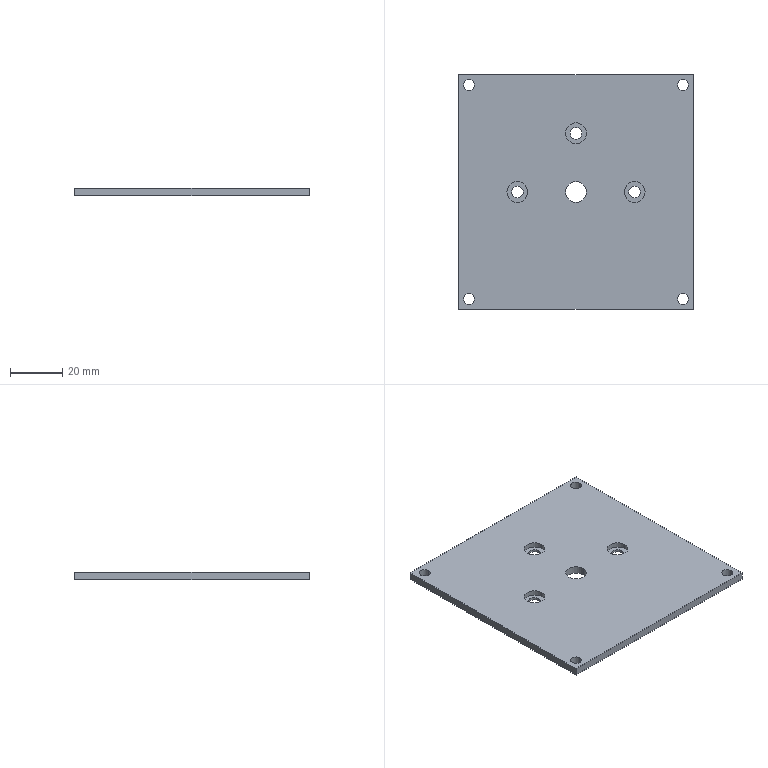Part | STEP file | output terminal base plate^spray gun PTFE model | 1 solid | 31 faces | box 90 x 90 x 3 mm | volume 23634 mm3 | cylinder 22 | plane 9 | commonest cylinder face diameters 4.2 x8 8 x8 4.5 x6
STEP:
#1=CARTESIAN_POINT('',(2.25,22.5,0.));
#2=VERTEX_POINT('',#1);
#3=CARTESIAN_POINT('',(-2.25,22.5,0.));
#4=VERTEX_POINT('',#3);
#5=CARTESIAN_POINT('',(0.,22.5,0.));
#6=DIRECTION('',(0.,0.,-1.));
#7=DIRECTION('',(1.,0.,0.));
#8=AXIS2_PLACEMENT_3D('',#5,#6,#7);
#9=CIRCLE('',#8,2.25);
#10=EDGE_CURVE('',#2,#4,#9,.T.);
#11=ORIENTED_EDGE('',*,*,#10,.T.);
#12=CARTESIAN_POINT('',(-2.25,22.5,1.));
#13=VERTEX_POINT('',#12);
#14=CARTESIAN_POINT('',(-2.25,22.5,-7.));
#15=DIRECTION('',(0.,0.,1.));
#16=VECTOR('',#15,1000.);
#17=LINE('',#14,#16);
#18=EDGE_CURVE('',#4,#13,#17,.T.);
#19=ORIENTED_EDGE('',*,*,#18,.T.);
#20=CARTESIAN_POINT('',(2.25,22.5,1.));
#21=VERTEX_POINT('',#20);
#22=CARTESIAN_POINT('',(0.,22.5,1.));
#23=DIRECTION('',(0.,0.,-1.));
#24=DIRECTION('',(1.,0.,0.));
#25=AXIS2_PLACEMENT_3D('',#22,#23,#24);
#26=CIRCLE('',#25,2.25);
#27=EDGE_CURVE('',#21,#13,#26,.T.);
#28=ORIENTED_EDGE('',*,*,#27,.F.);
#29=CARTESIAN_POINT('',(2.25,22.5,-7.));
#30=DIRECTION('',(0.,0.,1.));
#31=VECTOR('',#30,1000.);
#32=LINE('',#29,#31);
#33=EDGE_CURVE('',#2,#21,#32,.T.);
#34=ORIENTED_EDGE('',*,*,#33,.F.);
#35=EDGE_LOOP('',(#11,#19,#28,#34));
#36=FACE_OUTER_BOUND('',#35,.T.);
#37=CARTESIAN_POINT('',(0.,22.5,-7.));
#38=DIRECTION('',(0.,0.,1.));
#39=DIRECTION('',(1.,0.,0.));
#40=AXIS2_PLACEMENT_3D('',#37,#38,#39);
#41=CYLINDRICAL_SURFACE('',#40,2.25);
#42=ADVANCED_FACE('',(#36),#41,.F.);
#43=CARTESIAN_POINT('',(24.75,0.,0.));
#44=VERTEX_POINT('',#43);
#45=CARTESIAN_POINT('',(20.25,0.,0.));
#46=VERTEX_POINT('',#45);
#47=CARTESIAN_POINT('',(22.5,0.,0.));
#48=DIRECTION('',(0.,0.,-1.));
#49=DIRECTION('',(1.,0.,0.));
#50=AXIS2_PLACEMENT_3D('',#47,#48,#49);
#51=CIRCLE('',#50,2.25);
#52=EDGE_CURVE('',#44,#46,#51,.T.);
#53=ORIENTED_EDGE('',*,*,#52,.T.);
#54=CARTESIAN_POINT('',(20.25,0.,1.));
#55=VERTEX_POINT('',#54);
#56=CARTESIAN_POINT('',(20.25,0.,-7.));
#57=DIRECTION('',(0.,0.,1.));
#58=VECTOR('',#57,1000.);
#59=LINE('',#56,#58);
#60=EDGE_CURVE('',#46,#55,#59,.T.);
#61=ORIENTED_EDGE('',*,*,#60,.T.);
#62=CARTESIAN_POINT('',(24.75,0.,1.));
#63=VERTEX_POINT('',#62);
#64=CARTESIAN_POINT('',(22.5,0.,1.));
#65=DIRECTION('',(0.,0.,-1.));
#66=DIRECTION('',(1.,0.,0.));
#67=AXIS2_PLACEMENT_3D('',#64,#65,#66);
#68=CIRCLE('',#67,2.25);
#69=EDGE_CURVE('',#63,#55,#68,.T.);
#70=ORIENTED_EDGE('',*,*,#69,.F.);
#71=CARTESIAN_POINT('',(24.75,0.,-7.));
#72=DIRECTION('',(0.,0.,1.));
#73=VECTOR('',#72,1000.);
#74=LINE('',#71,#73);
#75=EDGE_CURVE('',#44,#63,#74,.T.);
#76=ORIENTED_EDGE('',*,*,#75,.F.);
#77=EDGE_LOOP('',(#53,#61,#70,#76));
#78=FACE_OUTER_BOUND('',#77,.T.);
#79=CARTESIAN_POINT('',(22.5,0.,-7.));
#80=DIRECTION('',(0.,0.,1.));
#81=DIRECTION('',(1.,0.,0.));
#82=AXIS2_PLACEMENT_3D('',#79,#80,#81);
#83=CYLINDRICAL_SURFACE('',#82,2.25);
#84=ADVANCED_FACE('',(#78),#83,.F.);
#85=CARTESIAN_POINT('',(-20.25,0.,0.));
#86=VERTEX_POINT('',#85);
#87=CARTESIAN_POINT('',(-24.75,0.,0.));
#88=VERTEX_POINT('',#87);
#89=CARTESIAN_POINT('',(-22.5,0.,0.));
#90=DIRECTION('',(0.,0.,-1.));
#91=DIRECTION('',(1.,0.,0.));
#92=AXIS2_PLACEMENT_3D('',#89,#90,#91);
#93=CIRCLE('',#92,2.25);
#94=EDGE_CURVE('',#86,#88,#93,.T.);
#95=ORIENTED_EDGE('',*,*,#94,.T.);
#96=CARTESIAN_POINT('',(-24.75,0.,1.));
#97=VERTEX_POINT('',#96);
#98=CARTESIAN_POINT('',(-24.75,0.,-7.));
#99=DIRECTION('',(0.,0.,1.));
#100=VECTOR('',#99,1000.);
#101=LINE('',#98,#100);
#102=EDGE_CURVE('',#88,#97,#101,.T.);
#103=ORIENTED_EDGE('',*,*,#102,.T.);
#104=CARTESIAN_POINT('',(-20.25,0.,1.));
#105=VERTEX_POINT('',#104);
#106=CARTESIAN_POINT('',(-22.5,0.,1.));
#107=DIRECTION('',(0.,0.,-1.));
#108=DIRECTION('',(1.,0.,0.));
#109=AXIS2_PLACEMENT_3D('',#106,#107,#108);
#110=CIRCLE('',#109,2.25);
#111=EDGE_CURVE('',#105,#97,#110,.T.);
#112=ORIENTED_EDGE('',*,*,#111,.F.);
#113=CARTESIAN_POINT('',(-20.25,0.,-7.));
#114=DIRECTION('',(0.,0.,1.));
#115=VECTOR('',#114,1000.);
#116=LINE('',#113,#115);
#117=EDGE_CURVE('',#86,#105,#116,.T.);
#118=ORIENTED_EDGE('',*,*,#117,.F.);
#119=EDGE_LOOP('',(#95,#103,#112,#118));
#120=FACE_OUTER_BOUND('',#119,.T.);
#121=CARTESIAN_POINT('',(-22.5,0.,-7.));
#122=DIRECTION('',(0.,0.,1.));
#123=DIRECTION('',(1.,0.,0.));
#124=AXIS2_PLACEMENT_3D('',#121,#122,#123);
#125=CYLINDRICAL_SURFACE('',#124,2.25);
#126=ADVANCED_FACE('',(#120),#125,.F.);
#127=CARTESIAN_POINT('',(43.1,-41.,3.));
#128=VERTEX_POINT('',#127);
#129=CARTESIAN_POINT('',(38.9,-41.,3.));
#130=VERTEX_POINT('',#129);
#131=CARTESIAN_POINT('',(41.,-41.,3.));
#132=DIRECTION('',(0.,0.,-1.));
#133=DIRECTION('',(-1.,0.,0.));
#134=AXIS2_PLACEMENT_3D('',#131,#132,#133);
#135=CIRCLE('',#134,2.1);
#136=EDGE_CURVE('',#128,#130,#135,.T.);
#137=ORIENTED_EDGE('',*,*,#136,.F.);
#138=CARTESIAN_POINT('',(43.1,-41.,0.));
#139=VERTEX_POINT('',#138);
#140=CARTESIAN_POINT('',(43.1,-41.,3.));
#141=DIRECTION('',(0.,0.,-1.));
#142=VECTOR('',#141,1000.);
#143=LINE('',#140,#142);
#144=EDGE_CURVE('',#128,#139,#143,.T.);
#145=ORIENTED_EDGE('',*,*,#144,.T.);
#146=CARTESIAN_POINT('',(38.9,-41.,0.));
#147=VERTEX_POINT('',#146);
#148=CARTESIAN_POINT('',(41.,-41.,0.));
#149=DIRECTION('',(0.,0.,-1.));
#150=DIRECTION('',(-1.,0.,0.));
#151=AXIS2_PLACEMENT_3D('',#148,#149,#150);
#152=CIRCLE('',#151,2.1);
#153=EDGE_CURVE('',#139,#147,#152,.T.);
#154=ORIENTED_EDGE('',*,*,#153,.T.);
#155=CARTESIAN_POINT('',(38.9,-41.,3.));
#156=DIRECTION('',(0.,0.,-1.));
#157=VECTOR('',#156,1000.);
#158=LINE('',#155,#157);
#159=EDGE_CURVE('',#130,#147,#158,.T.);
#160=ORIENTED_EDGE('',*,*,#159,.F.);
#161=EDGE_LOOP('',(#137,#145,#154,#160));
#162=FACE_OUTER_BOUND('',#161,.T.);
#163=CARTESIAN_POINT('',(41.,-41.,3.));
#164=DIRECTION('',(0.,0.,-1.));
#165=DIRECTION('',(-1.,0.,0.));
#166=AXIS2_PLACEMENT_3D('',#163,#164,#165);
#167=CYLINDRICAL_SURFACE('',#166,2.1);
#168=ADVANCED_FACE('',(#162),#167,.F.);
#169=CARTESIAN_POINT('',(43.1,41.,3.));
#170=VERTEX_POINT('',#169);
#171=CARTESIAN_POINT('',(38.9,41.,3.));
#172=VERTEX_POINT('',#171);
#173=CARTESIAN_POINT('',(41.,41.,3.));
#174=DIRECTION('',(0.,0.,-1.));
#175=DIRECTION('',(-1.,0.,0.));
#176=AXIS2_PLACEMENT_3D('',#173,#174,#175);
#177=CIRCLE('',#176,2.1);
#178=EDGE_CURVE('',#170,#172,#177,.T.);
#179=ORIENTED_EDGE('',*,*,#178,.F.);
#180=CARTESIAN_POINT('',(43.1,41.,0.));
#181=VERTEX_POINT('',#180);
#182=CARTESIAN_POINT('',(43.1,41.,3.));
#183=DIRECTION('',(0.,0.,-1.));
#184=VECTOR('',#183,1000.);
#185=LINE('',#182,#184);
#186=EDGE_CURVE('',#170,#181,#185,.T.);
#187=ORIENTED_EDGE('',*,*,#186,.T.);
#188=CARTESIAN_POINT('',(38.9,41.,0.));
#189=VERTEX_POINT('',#188);
#190=CARTESIAN_POINT('',(41.,41.,0.));
#191=DIRECTION('',(0.,0.,-1.));
#192=DIRECTION('',(-1.,0.,0.));
#193=AXIS2_PLACEMENT_3D('',#190,#191,#192);
#194=CIRCLE('',#193,2.1);
#195=EDGE_CURVE('',#181,#189,#194,.T.);
#196=ORIENTED_EDGE('',*,*,#195,.T.);
#197=CARTESIAN_POINT('',(38.9,41.,3.));
#198=DIRECTION('',(0.,0.,-1.));
#199=VECTOR('',#198,1000.);
#200=LINE('',#197,#199);
#201=EDGE_CURVE('',#172,#189,#200,.T.);
#202=ORIENTED_EDGE('',*,*,#201,.F.);
#203=EDGE_LOOP('',(#179,#187,#196,#202));
#204=FACE_OUTER_BOUND('',#203,.T.);
#205=CARTESIAN_POINT('',(41.,41.,3.));
#206=DIRECTION('',(0.,0.,-1.));
#207=DIRECTION('',(-1.,0.,0.));
#208=AXIS2_PLACEMENT_3D('',#205,#206,#207);
#209=CYLINDRICAL_SURFACE('',#208,2.1);
#210=ADVANCED_FACE('',(#204),#209,.F.);
#211=CARTESIAN_POINT('',(-38.9,41.,3.));
#212=VERTEX_POINT('',#211);
#213=CARTESIAN_POINT('',(-43.1,41.,3.));
#214=VERTEX_POINT('',#213);
#215=CARTESIAN_POINT('',(-41.,41.,3.));
#216=DIRECTION('',(0.,0.,-1.));
#217=DIRECTION('',(-1.,0.,0.));
#218=AXIS2_PLACEMENT_3D('',#215,#216,#217);
#219=CIRCLE('',#218,2.1);
#220=EDGE_CURVE('',#212,#214,#219,.T.);
#221=ORIENTED_EDGE('',*,*,#220,.F.);
#222=CARTESIAN_POINT('',(-38.9,41.,0.));
#223=VERTEX_POINT('',#222);
#224=CARTESIAN_POINT('',(-38.9,41.,3.));
#225=DIRECTION('',(0.,0.,-1.));
#226=VECTOR('',#225,1000.);
#227=LINE('',#224,#226);
#228=EDGE_CURVE('',#212,#223,#227,.T.);
#229=ORIENTED_EDGE('',*,*,#228,.T.);
#230=CARTESIAN_POINT('',(-43.1,41.,0.));
#231=VERTEX_POINT('',#230);
#232=CARTESIAN_POINT('',(-41.,41.,0.));
#233=DIRECTION('',(0.,0.,-1.));
#234=DIRECTION('',(-1.,0.,0.));
#235=AXIS2_PLACEMENT_3D('',#232,#233,#234);
#236=CIRCLE('',#235,2.1);
#237=EDGE_CURVE('',#223,#231,#236,.T.);
#238=ORIENTED_EDGE('',*,*,#237,.T.);
#239=CARTESIAN_POINT('',(-43.1,41.,3.));
#240=DIRECTION('',(0.,0.,-1.));
#241=VECTOR('',#240,1000.);
#242=LINE('',#239,#241);
#243=EDGE_CURVE('',#214,#231,#242,.T.);
#244=ORIENTED_EDGE('',*,*,#243,.F.);
#245=EDGE_LOOP('',(#221,#229,#238,#244));
#246=FACE_OUTER_BOUND('',#245,.T.);
#247=CARTESIAN_POINT('',(-41.,41.,3.));
#248=DIRECTION('',(0.,0.,-1.));
#249=DIRECTION('',(-1.,0.,0.));
#250=AXIS2_PLACEMENT_3D('',#247,#248,#249);
#251=CYLINDRICAL_SURFACE('',#250,2.1);
#252=ADVANCED_FACE('',(#246),#251,.F.);
#253=CARTESIAN_POINT('',(-38.9,-41.,3.));
#254=VERTEX_POINT('',#253);
#255=CARTESIAN_POINT('',(-43.1,-41.,3.));
#256=VERTEX_POINT('',#255);
#257=CARTESIAN_POINT('',(-41.,-41.,3.));
#258=DIRECTION('',(0.,0.,-1.));
#259=DIRECTION('',(-1.,0.,0.));
#260=AXIS2_PLACEMENT_3D('',#257,#258,#259);
#261=CIRCLE('',#260,2.1);
#262=EDGE_CURVE('',#254,#256,#261,.T.);
#263=ORIENTED_EDGE('',*,*,#262,.F.);
#264=CARTESIAN_POINT('',(-38.9,-41.,0.));
#265=VERTEX_POINT('',#264);
#266=CARTESIAN_POINT('',(-38.9,-41.,3.));
#267=DIRECTION('',(0.,0.,-1.));
#268=VECTOR('',#267,1000.);
#269=LINE('',#266,#268);
#270=EDGE_CURVE('',#254,#265,#269,.T.);
#271=ORIENTED_EDGE('',*,*,#270,.T.);
#272=CARTESIAN_POINT('',(-43.1,-41.,0.));
#273=VERTEX_POINT('',#272);
#274=CARTESIAN_POINT('',(-41.,-41.,0.));
#275=DIRECTION('',(0.,0.,-1.));
#276=DIRECTION('',(-1.,0.,0.));
#277=AXIS2_PLACEMENT_3D('',#274,#275,#276);
#278=CIRCLE('',#277,2.1);
#279=EDGE_CURVE('',#265,#273,#278,.T.);
#280=ORIENTED_EDGE('',*,*,#279,.T.);
#281=CARTESIAN_POINT('',(-43.1,-41.,3.));
#282=DIRECTION('',(0.,0.,-1.));
#283=VECTOR('',#282,1000.);
#284=LINE('',#281,#283);
#285=EDGE_CURVE('',#256,#273,#284,.T.);
#286=ORIENTED_EDGE('',*,*,#285,.F.);
#287=EDGE_LOOP('',(#263,#271,#280,#286));
#288=FACE_OUTER_BOUND('',#287,.T.);
#289=CARTESIAN_POINT('',(-41.,-41.,3.));
#290=DIRECTION('',(0.,0.,-1.));
#291=DIRECTION('',(-1.,0.,0.));
#292=AXIS2_PLACEMENT_3D('',#289,#290,#291);
#293=CYLINDRICAL_SURFACE('',#292,2.1);
#294=ADVANCED_FACE('',(#288),#293,.F.);
#295=CARTESIAN_POINT('',(4.,0.,3.));
#296=VERTEX_POINT('',#295);
#297=CARTESIAN_POINT('',(-4.,0.,3.));
#298=VERTEX_POINT('',#297);
#299=CARTESIAN_POINT('',(0.,0.,3.));
#300=DIRECTION('',(0.,0.,-1.));
#301=DIRECTION('',(-1.,0.,0.));
#302=AXIS2_PLACEMENT_3D('',#299,#300,#301);
#303=CIRCLE('',#302,4.);
#304=EDGE_CURVE('',#296,#298,#303,.T.);
#305=ORIENTED_EDGE('',*,*,#304,.F.);
#306=CARTESIAN_POINT('',(4.,0.,0.));
#307=VERTEX_POINT('',#306);
#308=CARTESIAN_POINT('',(4.,0.,3.));
#309=DIRECTION('',(0.,0.,-1.));
#310=VECTOR('',#309,1000.);
#311=LINE('',#308,#310);
#312=EDGE_CURVE('',#296,#307,#311,.T.);
#313=ORIENTED_EDGE('',*,*,#312,.T.);
#314=CARTESIAN_POINT('',(-4.,0.,0.));
#315=VERTEX_POINT('',#314);
#316=CARTESIAN_POINT('',(0.,0.,0.));
#317=DIRECTION('',(0.,0.,-1.));
#318=DIRECTION('',(-1.,0.,0.));
#319=AXIS2_PLACEMENT_3D('',#316,#317,#318);
#320=CIRCLE('',#319,4.);
#321=EDGE_CURVE('',#307,#315,#320,.T.);
#322=ORIENTED_EDGE('',*,*,#321,.T.);
#323=CARTESIAN_POINT('',(-4.,0.,3.));
#324=DIRECTION('',(0.,0.,-1.));
#325=VECTOR('',#324,1000.);
#326=LINE('',#323,#325);
#327=EDGE_CURVE('',#298,#315,#326,.T.);
#328=ORIENTED_EDGE('',*,*,#327,.F.);
#329=EDGE_LOOP('',(#305,#313,#322,#328));
#330=FACE_OUTER_BOUND('',#329,.T.);
#331=CARTESIAN_POINT('',(0.,0.,3.));
#332=DIRECTION('',(0.,0.,-1.));
#333=DIRECTION('',(-1.,0.,0.));
#334=AXIS2_PLACEMENT_3D('',#331,#332,#333);
#335=CYLINDRICAL_SURFACE('',#334,4.);
#336=ADVANCED_FACE('',(#330),#335,.F.);
#337=CARTESIAN_POINT('',(-4.,22.5,1.));
#338=VERTEX_POINT('',#337);
#339=CARTESIAN_POINT('',(4.,22.5,1.));
#340=VERTEX_POINT('',#339);
#341=CARTESIAN_POINT('',(0.,22.5,1.));
#342=DIRECTION('',(0.,0.,1.));
#343=DIRECTION('',(1.,0.,0.));
#344=AXIS2_PLACEMENT_3D('',#341,#342,#343);
#345=CIRCLE('',#344,4.);
#346=EDGE_CURVE('',#338,#340,#345,.T.);
#347=ORIENTED_EDGE('',*,*,#346,.F.);
#348=CARTESIAN_POINT('',(-4.,22.5,3.));
#349=VERTEX_POINT('',#348);
#350=CARTESIAN_POINT('',(-4.,22.5,1.));
#351=DIRECTION('',(0.,0.,1.));
#352=VECTOR('',#351,1000.);
#353=LINE('',#350,#352);
#354=EDGE_CURVE('',#338,#349,#353,.T.);
#355=ORIENTED_EDGE('',*,*,#354,.T.);
#356=CARTESIAN_POINT('',(4.,22.5,3.));
#357=VERTEX_POINT('',#356);
#358=CARTESIAN_POINT('',(0.,22.5,3.));
#359=DIRECTION('',(0.,0.,-1.));
#360=DIRECTION('',(1.,0.,0.));
#361=AXIS2_PLACEMENT_3D('',#358,#359,#360);
#362=CIRCLE('',#361,4.);
#363=EDGE_CURVE('',#357,#349,#362,.T.);
#364=ORIENTED_EDGE('',*,*,#363,.F.);
#365=CARTESIAN_POINT('',(4.,22.5,1.));
#366=DIRECTION('',(0.,0.,1.));
#367=VECTOR('',#366,1000.);
#368=LINE('',#365,#367);
#369=EDGE_CURVE('',#340,#357,#368,.T.);
#370=ORIENTED_EDGE('',*,*,#369,.F.);
#371=EDGE_LOOP('',(#347,#355,#364,#370));
#372=FACE_OUTER_BOUND('',#371,.T.);
#373=CARTESIAN_POINT('',(0.,22.5,1.));
#374=DIRECTION('',(0.,0.,1.));
#375=DIRECTION('',(1.,0.,0.));
#376=AXIS2_PLACEMENT_3D('',#373,#374,#375);
#377=CYLINDRICAL_SURFACE('',#376,4.);
#378=ADVANCED_FACE('',(#372),#377,.F.);
#379=CARTESIAN_POINT('',(18.5,0.,1.));
#380=VERTEX_POINT('',#379);
#381=CARTESIAN_POINT('',(26.5,0.,1.));
#382=VERTEX_POINT('',#381);
#383=CARTESIAN_POINT('',(22.5,0.,1.));
#384=DIRECTION('',(0.,0.,1.));
#385=DIRECTION('',(1.,0.,0.));
#386=AXIS2_PLACEMENT_3D('',#383,#384,#385);
#387=CIRCLE('',#386,4.);
#388=EDGE_CURVE('',#380,#382,#387,.T.);
#389=ORIENTED_EDGE('',*,*,#388,.F.);
#390=CARTESIAN_POINT('',(18.5,0.,3.));
#391=VERTEX_POINT('',#390);
#392=CARTESIAN_POINT('',(18.5,0.,1.));
#393=DIRECTION('',(0.,0.,1.));
#394=VECTOR('',#393,1000.);
#395=LINE('',#392,#394);
#396=EDGE_CURVE('',#380,#391,#395,.T.);
#397=ORIENTED_EDGE('',*,*,#396,.T.);
#398=CARTESIAN_POINT('',(26.5,0.,3.));
#399=VERTEX_POINT('',#398);
#400=CARTESIAN_POINT('',(22.5,0.,3.));
#401=DIRECTION('',(0.,0.,-1.));
#402=DIRECTION('',(1.,0.,0.));
#403=AXIS2_PLACEMENT_3D('',#400,#401,#402);
#404=CIRCLE('',#403,4.);
#405=EDGE_CURVE('',#399,#391,#404,.T.);
#406=ORIENTED_EDGE('',*,*,#405,.F.);
#407=CARTESIAN_POINT('',(26.5,0.,1.));
#408=DIRECTION('',(0.,0.,1.));
#409=VECTOR('',#408,1000.);
#410=LINE('',#407,#409);
#411=EDGE_CURVE('',#382,#399,#410,.T.);
#412=ORIENTED_EDGE('',*,*,#411,.F.);
#413=EDGE_LOOP('',(#389,#397,#406,#412));
#414=FACE_OUTER_BOUND('',#413,.T.);
#415=CARTESIAN_POINT('',(22.5,0.,1.));
#416=DIRECTION('',(0.,0.,1.));
#417=DIRECTION('',(1.,0.,0.));
#418=AXIS2_PLACEMENT_3D('',#415,#416,#417);
#419=CYLINDRICAL_SURFACE('',#418,4.);
#420=ADVANCED_FACE('',(#414),#419,.F.);
#421=CARTESIAN_POINT('',(-26.5,0.,1.));
#422=VERTEX_POINT('',#421);
#423=CARTESIAN_POINT('',(-18.5,0.,1.));
#424=VERTEX_POINT('',#423);
#425=CARTESIAN_POINT('',(-22.5,0.,1.));
#426=DIRECTION('',(0.,0.,1.));
#427=DIRECTION('',(1.,0.,0.));
#428=AXIS2_PLACEMENT_3D('',#425,#426,#427);
#429=CIRCLE('',#428,4.);
#430=EDGE_CURVE('',#422,#424,#429,.T.);
#431=ORIENTED_EDGE('',*,*,#430,.F.);
#432=CARTESIAN_POINT('',(-26.5,0.,3.));
#433=VERTEX_POINT('',#432);
#434=CARTESIAN_POINT('',(-26.5,0.,1.));
#435=DIRECTION('',(0.,0.,1.));
#436=VECTOR('',#435,1000.);
#437=LINE('',#434,#436);
#438=EDGE_CURVE('',#422,#433,#437,.T.);
#439=ORIENTED_EDGE('',*,*,#438,.T.);
#440=CARTESIAN_POINT('',(-18.5,0.,3.));
#441=VERTEX_POINT('',#440);
#442=CARTESIAN_POINT('',(-22.5,0.,3.));
#443=DIRECTION('',(0.,0.,-1.));
#444=DIRECTION('',(1.,0.,0.));
#445=AXIS2_PLACEMENT_3D('',#442,#443,#444);
#446=CIRCLE('',#445,4.);
#447=EDGE_CURVE('',#441,#433,#446,.T.);
#448=ORIENTED_EDGE('',*,*,#447,.F.);
#449=CARTESIAN_POINT('',(-18.5,0.,1.));
#450=DIRECTION('',(0.,0.,1.));
#451=VECTOR('',#450,1000.);
#452=LINE('',#449,#451);
#453=EDGE_CURVE('',#424,#441,#452,.T.);
#454=ORIENTED_EDGE('',*,*,#453,.F.);
#455=EDGE_LOOP('',(#431,#439,#448,#454));
#456=FACE_OUTER_BOUND('',#455,.T.);
#457=CARTESIAN_POINT('',(-22.5,0.,1.));
#458=DIRECTION('',(0.,0.,1.));
#459=DIRECTION('',(1.,0.,0.));
#460=AXIS2_PLACEMENT_3D('',#457,#458,#459);
#461=CYLINDRICAL_SURFACE('',#460,4.);
#462=ADVANCED_FACE('',(#456),#461,.F.);
#463=ORIENTED_EDGE('',*,*,#10,.F.);
#464=CARTESIAN_POINT('',(0.,22.5,0.));
#465=DIRECTION('',(0.,0.,-1.));
#466=DIRECTION('',(1.,0.,0.));
#467=AXIS2_PLACEMENT_3D('',#464,#465,#466);
#468=CIRCLE('',#467,2.25);
#469=EDGE_CURVE('',#4,#2,#468,.T.);
#470=ORIENTED_EDGE('',*,*,#469,.F.);
#471=EDGE_LOOP('',(#463,#470));
#472=FACE_BOUND('',#471,.T.);
#473=ORIENTED_EDGE('',*,*,#52,.F.);
#474=CARTESIAN_POINT('',(22.5,0.,0.));
#475=DIRECTION('',(0.,0.,-1.));
#476=DIRECTION('',(1.,0.,0.));
#477=AXIS2_PLACEMENT_3D('',#474,#475,#476);
#478=CIRCLE('',#477,2.25);
#479=EDGE_CURVE('',#46,#44,#478,.T.);
#480=ORIENTED_EDGE('',*,*,#479,.F.);
#481=EDGE_LOOP('',(#473,#480));
#482=FACE_BOUND('',#481,.T.);
#483=ORIENTED_EDGE('',*,*,#94,.F.);
#484=CARTESIAN_POINT('',(-22.5,0.,0.));
#485=DIRECTION('',(0.,0.,-1.));
#486=DIRECTION('',(1.,0.,0.));
#487=AXIS2_PLACEMENT_3D('',#484,#485,#486);
#488=CIRCLE('',#487,2.25);
#489=EDGE_CURVE('',#88,#86,#488,.T.);
#490=ORIENTED_EDGE('',*,*,#489,.F.);
#491=EDGE_LOOP('',(#483,#490));
#492=FACE_BOUND('',#491,.T.);
#493=CARTESIAN_POINT('',(41.,-41.,0.));
#494=DIRECTION('',(0.,0.,-1.));
#495=DIRECTION('',(-1.,0.,0.));
#496=AXIS2_PLACEMENT_3D('',#493,#494,#495);
#497=CIRCLE('',#496,2.1);
#498=EDGE_CURVE('',#147,#139,#497,.T.);
#499=ORIENTED_EDGE('',*,*,#498,.F.);
#500=ORIENTED_EDGE('',*,*,#153,.F.);
#501=EDGE_LOOP('',(#499,#500));
#502=FACE_BOUND('',#501,.T.);
#503=CARTESIAN_POINT('',(41.,41.,0.));
#504=DIRECTION('',(0.,0.,-1.));
#505=DIRECTION('',(-1.,0.,0.));
#506=AXIS2_PLACEMENT_3D('',#503,#504,#505);
#507=CIRCLE('',#506,2.1);
#508=EDGE_CURVE('',#189,#181,#507,.T.);
#509=ORIENTED_EDGE('',*,*,#508,.F.);
#510=ORIENTED_EDGE('',*,*,#195,.F.);
#511=EDGE_LOOP('',(#509,#510));
#512=FACE_BOUND('',#511,.T.);
#513=CARTESIAN_POINT('',(-45.,45.,0.));
#514=VERTEX_POINT('',#513);
#515=CARTESIAN_POINT('',(-45.,-45.,0.));
#516=VERTEX_POINT('',#515);
#517=CARTESIAN_POINT('',(-45.,0.,0.));
#518=DIRECTION('',(0.,-1.,0.));
#519=VECTOR('',#518,1000.);
#520=LINE('',#517,#519);
#521=EDGE_CURVE('',#514,#516,#520,.T.);
#522=ORIENTED_EDGE('',*,*,#521,.F.);
#523=CARTESIAN_POINT('',(45.,45.,0.));
#524=VERTEX_POINT('',#523);
#525=CARTESIAN_POINT('',(0.,45.,0.));
#526=DIRECTION('',(-1.,0.,0.));
#527=VECTOR('',#526,1000.);
#528=LINE('',#525,#527);
#529=EDGE_CURVE('',#524,#514,#528,.T.);
#530=ORIENTED_EDGE('',*,*,#529,.F.);
#531=CARTESIAN_POINT('',(45.,-45.,0.));
#532=VERTEX_POINT('',#531);
#533=CARTESIAN_POINT('',(45.,0.,0.));
#534=DIRECTION('',(0.,1.,0.));
#535=VECTOR('',#534,1000.);
#536=LINE('',#533,#535);
#537=EDGE_CURVE('',#532,#524,#536,.T.);
#538=ORIENTED_EDGE('',*,*,#537,.F.);
#539=CARTESIAN_POINT('',(0.,-45.,0.));
#540=DIRECTION('',(1.,0.,0.));
#541=VECTOR('',#540,1000.);
#542=LINE('',#539,#541);
#543=EDGE_CURVE('',#516,#532,#542,.T.);
#544=ORIENTED_EDGE('',*,*,#543,.F.);
#545=EDGE_LOOP('',(#522,#530,#538,#544));
#546=FACE_OUTER_BOUND('',#545,.T.);
#547=CARTESIAN_POINT('',(-41.,41.,0.));
#548=DIRECTION('',(0.,0.,-1.));
#549=DIRECTION('',(-1.,0.,0.));
#550=AXIS2_PLACEMENT_3D('',#547,#548,#549);
#551=CIRCLE('',#550,2.1);
#552=EDGE_CURVE('',#231,#223,#551,.T.);
#553=ORIENTED_EDGE('',*,*,#552,.F.);
#554=ORIENTED_EDGE('',*,*,#237,.F.);
#555=EDGE_LOOP('',(#553,#554));
#556=FACE_BOUND('',#555,.T.);
#557=CARTESIAN_POINT('',(-41.,-41.,0.));
#558=DIRECTION('',(0.,0.,-1.));
#559=DIRECTION('',(-1.,0.,0.));
#560=AXIS2_PLACEMENT_3D('',#557,#558,#559);
#561=CIRCLE('',#560,2.1);
#562=EDGE_CURVE('',#273,#265,#561,.T.);
#563=ORIENTED_EDGE('',*,*,#562,.F.);
#564=ORIENTED_EDGE('',*,*,#279,.F.);
#565=EDGE_LOOP('',(#563,#564));
#566=FACE_BOUND('',#565,.T.);
#567=CARTESIAN_POINT('',(0.,0.,0.));
#568=DIRECTION('',(0.,0.,-1.));
#569=DIRECTION('',(-1.,0.,0.));
#570=AXIS2_PLACEMENT_3D('',#567,#568,#569);
#571=CIRCLE('',#570,4.);
#572=EDGE_CURVE('',#315,#307,#571,.T.);
#573=ORIENTED_EDGE('',*,*,#572,.F.);
#574=ORIENTED_EDGE('',*,*,#321,.F.);
#575=EDGE_LOOP('',(#573,#574));
#576=FACE_BOUND('',#575,.T.);
#577=CARTESIAN_POINT('',(0.,0.,0.));
#578=DIRECTION('',(0.,0.,1.));
#579=DIRECTION('',(1.,0.,0.));
#580=AXIS2_PLACEMENT_3D('',#577,#578,#579);
#581=PLANE('',#580);
#582=ADVANCED_FACE('',(#472,#482,#492,#502,#512,#546,#556,#566,#576),#581,.F.);
#583=ORIENTED_EDGE('',*,*,#18,.F.);
#584=ORIENTED_EDGE('',*,*,#469,.T.);
#585=ORIENTED_EDGE('',*,*,#33,.T.);
#586=CARTESIAN_POINT('',(0.,22.5,1.));
#587=DIRECTION('',(0.,0.,-1.));
#588=DIRECTION('',(1.,0.,0.));
#589=AXIS2_PLACEMENT_3D('',#586,#587,#588);
#590=CIRCLE('',#589,2.25);
#591=EDGE_CURVE('',#13,#21,#590,.T.);
#592=ORIENTED_EDGE('',*,*,#591,.F.);
#593=EDGE_LOOP('',(#583,#584,#585,#592));
#594=FACE_OUTER_BOUND('',#593,.T.);
#595=CARTESIAN_POINT('',(0.,22.5,-7.));
#596=DIRECTION('',(0.,0.,1.));
#597=DIRECTION('',(1.,0.,0.));
#598=AXIS2_PLACEMENT_3D('',#595,#596,#597);
#599=CYLINDRICAL_SURFACE('',#598,2.25);
#600=ADVANCED_FACE('',(#594),#599,.F.);
#601=ORIENTED_EDGE('',*,*,#60,.F.);
#602=ORIENTED_EDGE('',*,*,#479,.T.);
#603=ORIENTED_EDGE('',*,*,#75,.T.);
#604=CARTESIAN_POINT('',(22.5,0.,1.));
#605=DIRECTION('',(0.,0.,-1.));
#606=DIRECTION('',(1.,0.,0.));
#607=AXIS2_PLACEMENT_3D('',#604,#605,#606);
#608=CIRCLE('',#607,2.25);
#609=EDGE_CURVE('',#55,#63,#608,.T.);
#610=ORIENTED_EDGE('',*,*,#609,.F.);
#611=EDGE_LOOP('',(#601,#602,#603,#610));
#612=FACE_OUTER_BOUND('',#611,.T.);
#613=CARTESIAN_POINT('',(22.5,0.,-7.));
#614=DIRECTION('',(0.,0.,1.));
#615=DIRECTION('',(1.,0.,0.));
#616=AXIS2_PLACEMENT_3D('',#613,#614,#615);
#617=CYLINDRICAL_SURFACE('',#616,2.25);
#618=ADVANCED_FACE('',(#612),#617,.F.);
#619=ORIENTED_EDGE('',*,*,#102,.F.);
#620=ORIENTED_EDGE('',*,*,#489,.T.);
#621=ORIENTED_EDGE('',*,*,#117,.T.);
#622=CARTESIAN_POINT('',(-22.5,0.,1.));
#623=DIRECTION('',(0.,0.,-1.));
#624=DIRECTION('',(1.,0.,0.));
#625=AXIS2_PLACEMENT_3D('',#622,#623,#624);
#626=CIRCLE('',#625,2.25);
#627=EDGE_CURVE('',#97,#105,#626,.T.);
#628=ORIENTED_EDGE('',*,*,#627,.F.);
#629=EDGE_LOOP('',(#619,#620,#621,#628));
#630=FACE_OUTER_BOUND('',#629,.T.);
#631=CARTESIAN_POINT('',(-22.5,0.,-7.));
#632=DIRECTION('',(0.,0.,1.));
#633=DIRECTION('',(1.,0.,0.));
#634=AXIS2_PLACEMENT_3D('',#631,#632,#633);
#635=CYLINDRICAL_SURFACE('',#634,2.25);
#636=ADVANCED_FACE('',(#630),#635,.F.);
#637=ORIENTED_EDGE('',*,*,#144,.F.);
#638=CARTESIAN_POINT('',(41.,-41.,3.));
#639=DIRECTION('',(0.,0.,-1.));
#640=DIRECTION('',(-1.,0.,0.));
#641=AXIS2_PLACEMENT_3D('',#638,#639,#640);
#642=CIRCLE('',#641,2.1);
#643=EDGE_CURVE('',#130,#128,#642,.T.);
#644=ORIENTED_EDGE('',*,*,#643,.F.);
#645=ORIENTED_EDGE('',*,*,#159,.T.);
#646=ORIENTED_EDGE('',*,*,#498,.T.);
#647=EDGE_LOOP('',(#637,#644,#645,#646));
#648=FACE_OUTER_BOUND('',#647,.T.);
#649=CARTESIAN_POINT('',(41.,-41.,3.));
#650=DIRECTION('',(0.,0.,-1.));
#651=DIRECTION('',(-1.,0.,0.));
#652=AXIS2_PLACEMENT_3D('',#649,#650,#651);
#653=CYLINDRICAL_SURFACE('',#652,2.1);
#654=ADVANCED_FACE('',(#648),#653,.F.);
#655=ORIENTED_EDGE('',*,*,#186,.F.);
#656=CARTESIAN_POINT('',(41.,41.,3.));
#657=DIRECTION('',(0.,0.,-1.));
#658=DIRECTION('',(-1.,0.,0.));
#659=AXIS2_PLACEMENT_3D('',#656,#657,#658);
#660=CIRCLE('',#659,2.1);
#661=EDGE_CURVE('',#172,#170,#660,.T.);
#662=ORIENTED_EDGE('',*,*,#661,.F.);
#663=ORIENTED_EDGE('',*,*,#201,.T.);
#664=ORIENTED_EDGE('',*,*,#508,.T.);
#665=EDGE_LOOP('',(#655,#662,#663,#664));
#666=FACE_OUTER_BOUND('',#665,.T.);
#667=CARTESIAN_POINT('',(41.,41.,3.));
#668=DIRECTION('',(0.,0.,-1.));
#669=DIRECTION('',(-1.,0.,0.));
#670=AXIS2_PLACEMENT_3D('',#667,#668,#669);
#671=CYLINDRICAL_SURFACE('',#670,2.1);
#672=ADVANCED_FACE('',(#666),#671,.F.);
#673=CARTESIAN_POINT('',(-45.,-45.,3.));
#674=VERTEX_POINT('',#673);
#675=CARTESIAN_POINT('',(45.,-45.,3.));
#676=VERTEX_POINT('',#675);
#677=CARTESIAN_POINT('',(-45.,-45.,3.));
#678=DIRECTION('',(1.,0.,0.));
#679=VECTOR('',#678,1000.);
#680=LINE('',#677,#679);
#681=EDGE_CURVE('',#674,#676,#680,.T.);
#682=ORIENTED_EDGE('',*,*,#681,.F.);
#683=CARTESIAN_POINT('',(-45.,-45.,3.));
#684=DIRECTION('',(0.,0.,1.));
#685=VECTOR('',#684,1000.);
#686=LINE('',#683,#685);
#687=EDGE_CURVE('',#516,#674,#686,.T.);
#688=ORIENTED_EDGE('',*,*,#687,.F.);
#689=ORIENTED_EDGE('',*,*,#543,.T.);
#690=CARTESIAN_POINT('',(45.,-45.,3.));
#691=DIRECTION('',(0.,0.,-1.));
#692=VECTOR('',#691,1000.);
#693=LINE('',#690,#692);
#694=EDGE_CURVE('',#676,#532,#693,.T.);
#695=ORIENTED_EDGE('',*,*,#694,.F.);
#696=EDGE_LOOP('',(#682,#688,#689,#695));
#697=FACE_OUTER_BOUND('',#696,.T.);
#698=CARTESIAN_POINT('',(-45.,-45.,3.));
#699=DIRECTION('',(0.,1.,0.));
#700=DIRECTION('',(0.,0.,1.));
#701=AXIS2_PLACEMENT_3D('',#698,#699,#700);
#702=PLANE('',#701);
#703=ADVANCED_FACE('',(#697),#702,.F.);
#704=CARTESIAN_POINT('',(-45.,45.,3.));
#705=VERTEX_POINT('',#704);
#706=CARTESIAN_POINT('',(-45.,45.,3.));
#707=DIRECTION('',(0.,-1.,0.));
#708=VECTOR('',#707,1000.);
#709=LINE('',#706,#708);
#710=EDGE_CURVE('',#705,#674,#709,.T.);
#711=ORIENTED_EDGE('',*,*,#710,.F.);
#712=CARTESIAN_POINT('',(-45.,45.,3.));
#713=DIRECTION('',(0.,0.,1.));
#714=VECTOR('',#713,1000.);
#715=LINE('',#712,#714);
#716=EDGE_CURVE('',#514,#705,#715,.T.);
#717=ORIENTED_EDGE('',*,*,#716,.F.);
#718=ORIENTED_EDGE('',*,*,#521,.T.);
#719=ORIENTED_EDGE('',*,*,#687,.T.);
#720=EDGE_LOOP('',(#711,#717,#718,#719));
#721=FACE_OUTER_BOUND('',#720,.T.);
#722=CARTESIAN_POINT('',(-45.,45.,3.));
#723=DIRECTION('',(1.,0.,0.));
#724=DIRECTION('',(0.,1.,0.));
#725=AXIS2_PLACEMENT_3D('',#722,#723,#724);
#726=PLANE('',#725);
#727=ADVANCED_FACE('',(#721),#726,.F.);
#728=CARTESIAN_POINT('',(45.,45.,3.));
#729=VERTEX_POINT('',#728);
#730=CARTESIAN_POINT('',(-45.,45.,3.));
#731=DIRECTION('',(-1.,0.,0.));
#732=VECTOR('',#731,1000.);
#733=LINE('',#730,#732);
#734=EDGE_CURVE('',#729,#705,#733,.T.);
#735=ORIENTED_EDGE('',*,*,#734,.F.);
#736=CARTESIAN_POINT('',(45.,45.,3.));
#737=DIRECTION('',(0.,0.,1.));
#738=VECTOR('',#737,1000.);
#739=LINE('',#736,#738);
#740=EDGE_CURVE('',#524,#729,#739,.T.);
#741=ORIENTED_EDGE('',*,*,#740,.F.);
#742=ORIENTED_EDGE('',*,*,#529,.T.);
#743=ORIENTED_EDGE('',*,*,#716,.T.);
#744=EDGE_LOOP('',(#735,#741,#742,#743));
#745=FACE_OUTER_BOUND('',#744,.T.);
#746=CARTESIAN_POINT('',(-45.,45.,3.));
#747=DIRECTION('',(0.,-1.,0.));
#748=DIRECTION('',(0.,0.,-1.));
#749=AXIS2_PLACEMENT_3D('',#746,#747,#748);
#750=PLANE('',#749);
#751=ADVANCED_FACE('',(#745),#750,.F.);
#752=CARTESIAN_POINT('',(45.,45.,3.));
#753=DIRECTION('',(0.,1.,0.));
#754=VECTOR('',#753,1000.);
#755=LINE('',#752,#754);
#756=EDGE_CURVE('',#676,#729,#755,.T.);
#757=ORIENTED_EDGE('',*,*,#756,.F.);
#758=ORIENTED_EDGE('',*,*,#694,.T.);
#759=ORIENTED_EDGE('',*,*,#537,.T.);
#760=ORIENTED_EDGE('',*,*,#740,.T.);
#761=EDGE_LOOP('',(#757,#758,#759,#760));
#762=FACE_OUTER_BOUND('',#761,.T.);
#763=CARTESIAN_POINT('',(45.,45.,3.));
#764=DIRECTION('',(-1.,0.,0.));
#765=DIRECTION('',(0.,-1.,0.));
#766=AXIS2_PLACEMENT_3D('',#763,#764,#765);
#767=PLANE('',#766);
#768=ADVANCED_FACE('',(#762),#767,.F.);
#769=ORIENTED_EDGE('',*,*,#228,.F.);
#770=CARTESIAN_POINT('',(-41.,41.,3.));
#771=DIRECTION('',(0.,0.,-1.));
#772=DIRECTION('',(-1.,0.,0.));
#773=AXIS2_PLACEMENT_3D('',#770,#771,#772);
#774=CIRCLE('',#773,2.1);
#775=EDGE_CURVE('',#214,#212,#774,.T.);
#776=ORIENTED_EDGE('',*,*,#775,.F.);
#777=ORIENTED_EDGE('',*,*,#243,.T.);
#778=ORIENTED_EDGE('',*,*,#552,.T.);
#779=EDGE_LOOP('',(#769,#776,#777,#778));
#780=FACE_OUTER_BOUND('',#779,.T.);
#781=CARTESIAN_POINT('',(-41.,41.,3.));
#782=DIRECTION('',(0.,0.,-1.));
#783=DIRECTION('',(-1.,0.,0.));
#784=AXIS2_PLACEMENT_3D('',#781,#782,#783);
#785=CYLINDRICAL_SURFACE('',#784,2.1);
#786=ADVANCED_FACE('',(#780),#785,.F.);
#787=ORIENTED_EDGE('',*,*,#270,.F.);
#788=CARTESIAN_POINT('',(-41.,-41.,3.));
#789=DIRECTION('',(0.,0.,-1.));
#790=DIRECTION('',(-1.,0.,0.));
#791=AXIS2_PLACEMENT_3D('',#788,#789,#790);
#792=CIRCLE('',#791,2.1);
#793=EDGE_CURVE('',#256,#254,#792,.T.);
#794=ORIENTED_EDGE('',*,*,#793,.F.);
#795=ORIENTED_EDGE('',*,*,#285,.T.);
#796=ORIENTED_EDGE('',*,*,#562,.T.);
#797=EDGE_LOOP('',(#787,#794,#795,#796));
#798=FACE_OUTER_BOUND('',#797,.T.);
#799=CARTESIAN_POINT('',(-41.,-41.,3.));
#800=DIRECTION('',(0.,0.,-1.));
#801=DIRECTION('',(-1.,0.,0.));
#802=AXIS2_PLACEMENT_3D('',#799,#800,#801);
#803=CYLINDRICAL_SURFACE('',#802,2.1);
#804=ADVANCED_FACE('',(#798),#803,.F.);
#805=ORIENTED_EDGE('',*,*,#312,.F.);
#806=CARTESIAN_POINT('',(0.,0.,3.));
#807=DIRECTION('',(0.,0.,-1.));
#808=DIRECTION('',(-1.,0.,0.));
#809=AXIS2_PLACEMENT_3D('',#806,#807,#808);
#810=CIRCLE('',#809,4.);
#811=EDGE_CURVE('',#298,#296,#810,.T.);
#812=ORIENTED_EDGE('',*,*,#811,.F.);
#813=ORIENTED_EDGE('',*,*,#327,.T.);
#814=ORIENTED_EDGE('',*,*,#572,.T.);
#815=EDGE_LOOP('',(#805,#812,#813,#814));
#816=FACE_OUTER_BOUND('',#815,.T.);
#817=CARTESIAN_POINT('',(0.,0.,3.));
#818=DIRECTION('',(0.,0.,-1.));
#819=DIRECTION('',(-1.,0.,0.));
#820=AXIS2_PLACEMENT_3D('',#817,#818,#819);
#821=CYLINDRICAL_SURFACE('',#820,4.);
#822=ADVANCED_FACE('',(#816),#821,.F.);
#823=CARTESIAN_POINT('',(0.,22.5,1.));
#824=DIRECTION('',(0.,0.,1.));
#825=DIRECTION('',(1.,0.,0.));
#826=AXIS2_PLACEMENT_3D('',#823,#824,#825);
#827=CIRCLE('',#826,4.);
#828=EDGE_CURVE('',#340,#338,#827,.T.);
#829=ORIENTED_EDGE('',*,*,#828,.T.);
#830=ORIENTED_EDGE('',*,*,#346,.T.);
#831=EDGE_LOOP('',(#829,#830));
#832=FACE_OUTER_BOUND('',#831,.T.);
#833=ORIENTED_EDGE('',*,*,#27,.T.);
#834=ORIENTED_EDGE('',*,*,#591,.T.);
#835=EDGE_LOOP('',(#833,#834));
#836=FACE_BOUND('',#835,.T.);
#837=CARTESIAN_POINT('',(0.,22.5,1.));
#838=DIRECTION('',(0.,0.,1.));
#839=DIRECTION('',(1.,0.,0.));
#840=AXIS2_PLACEMENT_3D('',#837,#838,#839);
#841=PLANE('',#840);
#842=ADVANCED_FACE('',(#832,#836),#841,.T.);
#843=CARTESIAN_POINT('',(22.5,0.,1.));
#844=DIRECTION('',(0.,0.,1.));
#845=DIRECTION('',(1.,0.,0.));
#846=AXIS2_PLACEMENT_3D('',#843,#844,#845);
#847=CIRCLE('',#846,4.);
#848=EDGE_CURVE('',#382,#380,#847,.T.);
#849=ORIENTED_EDGE('',*,*,#848,.T.);
#850=ORIENTED_EDGE('',*,*,#388,.T.);
#851=EDGE_LOOP('',(#849,#850));
#852=FACE_OUTER_BOUND('',#851,.T.);
#853=ORIENTED_EDGE('',*,*,#69,.T.);
#854=ORIENTED_EDGE('',*,*,#609,.T.);
#855=EDGE_LOOP('',(#853,#854));
#856=FACE_BOUND('',#855,.T.);
#857=CARTESIAN_POINT('',(22.5,0.,1.));
#858=DIRECTION('',(0.,0.,1.));
#859=DIRECTION('',(1.,0.,0.));
#860=AXIS2_PLACEMENT_3D('',#857,#858,#859);
#861=PLANE('',#860);
#862=ADVANCED_FACE('',(#852,#856),#861,.T.);
#863=CARTESIAN_POINT('',(-22.5,0.,1.));
#864=DIRECTION('',(0.,0.,1.));
#865=DIRECTION('',(1.,0.,0.));
#866=AXIS2_PLACEMENT_3D('',#863,#864,#865);
#867=CIRCLE('',#866,4.);
#868=EDGE_CURVE('',#424,#422,#867,.T.);
#869=ORIENTED_EDGE('',*,*,#868,.T.);
#870=ORIENTED_EDGE('',*,*,#430,.T.);
#871=EDGE_LOOP('',(#869,#870));
#872=FACE_OUTER_BOUND('',#871,.T.);
#873=ORIENTED_EDGE('',*,*,#111,.T.);
#874=ORIENTED_EDGE('',*,*,#627,.T.);
#875=EDGE_LOOP('',(#873,#874));
#876=FACE_BOUND('',#875,.T.);
#877=CARTESIAN_POINT('',(-22.5,0.,1.));
#878=DIRECTION('',(0.,0.,1.));
#879=DIRECTION('',(1.,0.,0.));
#880=AXIS2_PLACEMENT_3D('',#877,#878,#879);
#881=PLANE('',#880);
#882=ADVANCED_FACE('',(#872,#876),#881,.T.);
#883=ORIENTED_EDGE('',*,*,#405,.T.);
#884=CARTESIAN_POINT('',(22.5,0.,3.));
#885=DIRECTION('',(0.,0.,-1.));
#886=DIRECTION('',(1.,0.,0.));
#887=AXIS2_PLACEMENT_3D('',#884,#885,#886);
#888=CIRCLE('',#887,4.);
#889=EDGE_CURVE('',#391,#399,#888,.T.);
#890=ORIENTED_EDGE('',*,*,#889,.T.);
#891=EDGE_LOOP('',(#883,#890));
#892=FACE_BOUND('',#891,.T.);
#893=ORIENTED_EDGE('',*,*,#447,.T.);
#894=CARTESIAN_POINT('',(-22.5,0.,3.));
#895=DIRECTION('',(0.,0.,-1.));
#896=DIRECTION('',(1.,0.,0.));
#897=AXIS2_PLACEMENT_3D('',#894,#895,#896);
#898=CIRCLE('',#897,4.);
#899=EDGE_CURVE('',#433,#441,#898,.T.);
#900=ORIENTED_EDGE('',*,*,#899,.T.);
#901=EDGE_LOOP('',(#893,#900));
#902=FACE_BOUND('',#901,.T.);
#903=ORIENTED_EDGE('',*,*,#363,.T.);
#904=CARTESIAN_POINT('',(0.,22.5,3.));
#905=DIRECTION('',(0.,0.,-1.));
#906=DIRECTION('',(1.,0.,0.));
#907=AXIS2_PLACEMENT_3D('',#904,#905,#906);
#908=CIRCLE('',#907,4.);
#909=EDGE_CURVE('',#349,#357,#908,.T.);
#910=ORIENTED_EDGE('',*,*,#909,.T.);
#911=EDGE_LOOP('',(#903,#910));
#912=FACE_BOUND('',#911,.T.);
#913=ORIENTED_EDGE('',*,*,#643,.T.);
#914=ORIENTED_EDGE('',*,*,#136,.T.);
#915=EDGE_LOOP('',(#913,#914));
#916=FACE_BOUND('',#915,.T.);
#917=ORIENTED_EDGE('',*,*,#661,.T.);
#918=ORIENTED_EDGE('',*,*,#178,.T.);
#919=EDGE_LOOP('',(#917,#918));
#920=FACE_BOUND('',#919,.T.);
#921=ORIENTED_EDGE('',*,*,#756,.T.);
#922=ORIENTED_EDGE('',*,*,#734,.T.);
#923=ORIENTED_EDGE('',*,*,#710,.T.);
#924=ORIENTED_EDGE('',*,*,#681,.T.);
#925=EDGE_LOOP('',(#921,#922,#923,#924));
#926=FACE_OUTER_BOUND('',#925,.T.);
#927=ORIENTED_EDGE('',*,*,#775,.T.);
#928=ORIENTED_EDGE('',*,*,#220,.T.);
#929=EDGE_LOOP('',(#927,#928));
#930=FACE_BOUND('',#929,.T.);
#931=ORIENTED_EDGE('',*,*,#793,.T.);
#932=ORIENTED_EDGE('',*,*,#262,.T.);
#933=EDGE_LOOP('',(#931,#932));
#934=FACE_BOUND('',#933,.T.);
#935=ORIENTED_EDGE('',*,*,#811,.T.);
#936=ORIENTED_EDGE('',*,*,#304,.T.);
#937=EDGE_LOOP('',(#935,#936));
#938=FACE_BOUND('',#937,.T.);
#939=CARTESIAN_POINT('',(0.,0.,3.));
#940=DIRECTION('',(0.,0.,1.));
#941=DIRECTION('',(1.,0.,0.));
#942=AXIS2_PLACEMENT_3D('',#939,#940,#941);
#943=PLANE('',#942);
#944=ADVANCED_FACE('',(#892,#902,#912,#916,#920,#926,#930,#934,#938),#943,.T.);
#945=ORIENTED_EDGE('',*,*,#354,.F.);
#946=ORIENTED_EDGE('',*,*,#828,.F.);
#947=ORIENTED_EDGE('',*,*,#369,.T.);
#948=ORIENTED_EDGE('',*,*,#909,.F.);
#949=EDGE_LOOP('',(#945,#946,#947,#948));
#950=FACE_OUTER_BOUND('',#949,.T.);
#951=CARTESIAN_POINT('',(0.,22.5,1.));
#952=DIRECTION('',(0.,0.,1.));
#953=DIRECTION('',(1.,0.,0.));
#954=AXIS2_PLACEMENT_3D('',#951,#952,#953);
#955=CYLINDRICAL_SURFACE('',#954,4.);
#956=ADVANCED_FACE('',(#950),#955,.F.);
#957=ORIENTED_EDGE('',*,*,#396,.F.);
#958=ORIENTED_EDGE('',*,*,#848,.F.);
#959=ORIENTED_EDGE('',*,*,#411,.T.);
#960=ORIENTED_EDGE('',*,*,#889,.F.);
#961=EDGE_LOOP('',(#957,#958,#959,#960));
#962=FACE_OUTER_BOUND('',#961,.T.);
#963=CARTESIAN_POINT('',(22.5,0.,1.));
#964=DIRECTION('',(0.,0.,1.));
#965=DIRECTION('',(1.,0.,0.));
#966=AXIS2_PLACEMENT_3D('',#963,#964,#965);
#967=CYLINDRICAL_SURFACE('',#966,4.);
#968=ADVANCED_FACE('',(#962),#967,.F.);
#969=ORIENTED_EDGE('',*,*,#438,.F.);
#970=ORIENTED_EDGE('',*,*,#868,.F.);
#971=ORIENTED_EDGE('',*,*,#453,.T.);
#972=ORIENTED_EDGE('',*,*,#899,.F.);
#973=EDGE_LOOP('',(#969,#970,#971,#972));
#974=FACE_OUTER_BOUND('',#973,.T.);
#975=CARTESIAN_POINT('',(-22.5,0.,1.));
#976=DIRECTION('',(0.,0.,1.));
#977=DIRECTION('',(1.,0.,0.));
#978=AXIS2_PLACEMENT_3D('',#975,#976,#977);
#979=CYLINDRICAL_SURFACE('',#978,4.);
#980=ADVANCED_FACE('',(#974),#979,.F.);
#981=CLOSED_SHELL('',(#42,#84,#126,#168,#210,#252,#294,#336,#378,#420,#462,#582,#600,#618,#636,#654,#672,#703,#727,#751,#768,#786,#804,#822,#842,#862,#882,#944,#956,#968,#980));
#982=MANIFOLD_SOLID_BREP('',#981);
#983=CARTESIAN_POINT('',(0.,0.,0.));
#984=DIRECTION('',(0.,0.,1.));
#985=DIRECTION('',(1.,0.,0.));
#986=AXIS2_PLACEMENT_3D('',#983,#984,#985);
#987=(LENGTH_UNIT()NAMED_UNIT(*)SI_UNIT(.MILLI.,.METRE.));
#988=UNCERTAINTY_MEASURE_WITH_UNIT(LENGTH_MEASURE(0.00001),#987,'','');
#989=(NAMED_UNIT(*)PLANE_ANGLE_UNIT()SI_UNIT($,.RADIAN.));
#990=(NAMED_UNIT(*)SI_UNIT($,.STERADIAN.)SOLID_ANGLE_UNIT());
#991=(GEOMETRIC_REPRESENTATION_CONTEXT(3)GLOBAL_UNCERTAINTY_ASSIGNED_CONTEXT((#988))GLOBAL_UNIT_ASSIGNED_CONTEXT((#987,#989,#990))REPRESENTATION_CONTEXT('',''));
#992=ADVANCED_BREP_SHAPE_REPRESENTATION('',(#982,#986),#991);